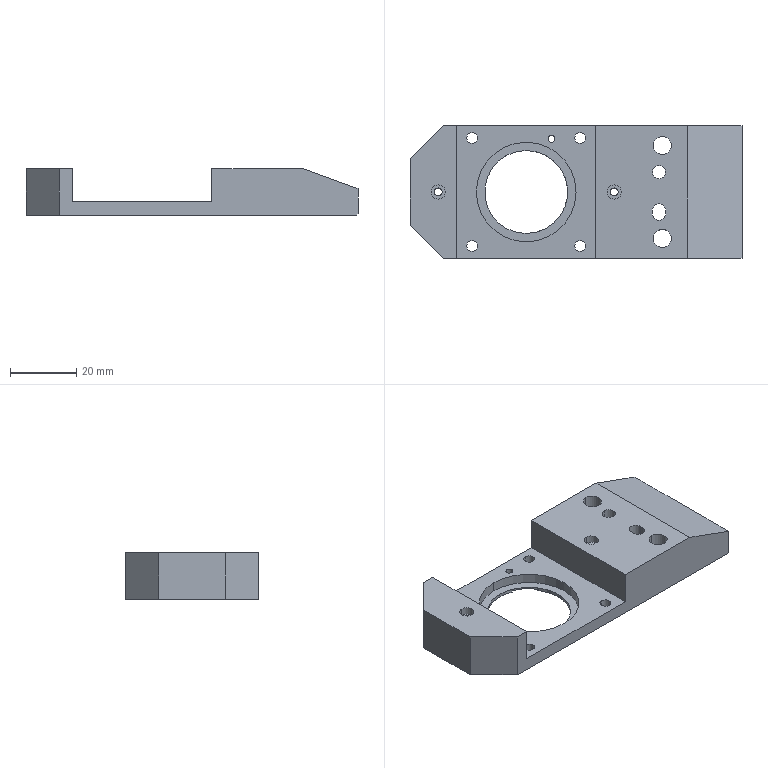NC program | NX | posted with a generic post | part box 100 x 40 x 14 mm
Lines 1 to 18 of 15435:
N10 G17 G21 G94 G90
(FLOOR_WALL_COPY , TOOL : D50R0.8)
N12 T03 M6
N14 G54
N16 G17 G0 G90 X-81. Y0. S1500 M3
N18 G43 Z30. H3
N20 Z3.
N22 G94 G1 Z0. F1000.
N24 X-78.
N26 X78.
N28 X81.
N30 Z3.
N32 G0 Z30.
N34 M5